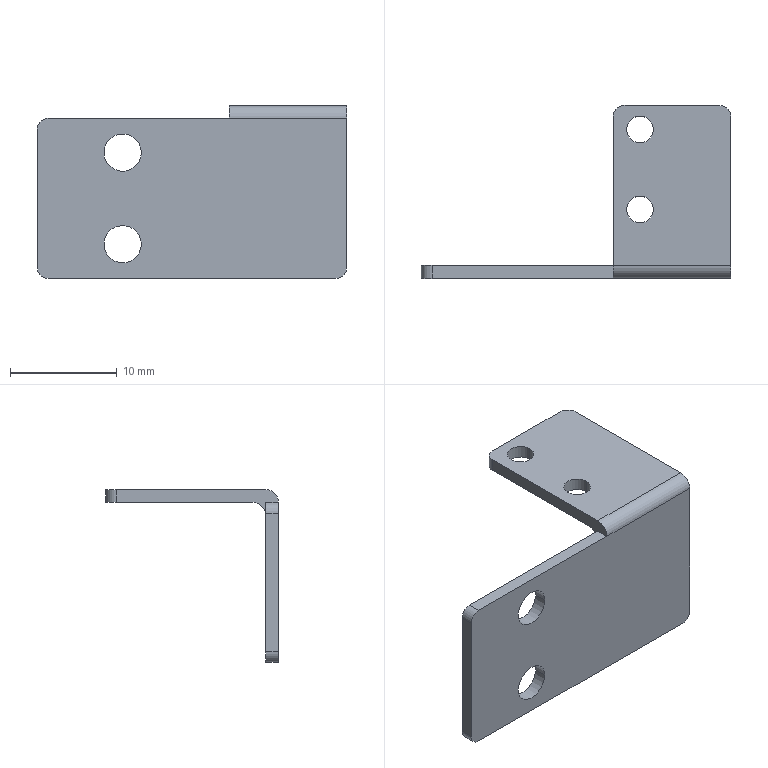Part | STEP file | 11-FG-B01311 | 1 solid | 25 faces | box 29 x 16.2 x 16.2 mm | volume 699.681 mm3 | cylinder 15 | plane 10 | commonest cylinder face diameters 2 x5 2.5 x4 3.5 x4 2.4 x2
STEP:
#1=CARTESIAN_POINT('',(-19.25,0.,-3.2));
#2=VERTEX_POINT('',#1);
#3=CARTESIAN_POINT('',(-22.75,0.,-3.2));
#4=VERTEX_POINT('',#3);
#5=CARTESIAN_POINT('',(-21.,0.,-3.2));
#6=DIRECTION('',(0.,1.,0.));
#7=DIRECTION('',(0.,0.,1.));
#8=AXIS2_PLACEMENT_3D('',#5,#6,#7);
#9=CIRCLE('',#8,1.75);
#10=EDGE_CURVE('',#2,#4,#9,.T.);
#11=ORIENTED_EDGE('',*,*,#10,.F.);
#12=CARTESIAN_POINT('',(-19.25,1.2,-3.2));
#13=VERTEX_POINT('',#12);
#14=CARTESIAN_POINT('',(-19.25,-8.8,-3.2));
#15=DIRECTION('',(0.,1.,0.));
#16=VECTOR('',#15,1000.);
#17=LINE('',#14,#16);
#18=EDGE_CURVE('',#2,#13,#17,.T.);
#19=ORIENTED_EDGE('',*,*,#18,.T.);
#20=CARTESIAN_POINT('',(-22.75,1.2,-3.2));
#21=VERTEX_POINT('',#20);
#22=CARTESIAN_POINT('',(-21.,1.2,-3.2));
#23=DIRECTION('',(0.,1.,0.));
#24=DIRECTION('',(-1.,0.,0.));
#25=AXIS2_PLACEMENT_3D('',#22,#23,#24);
#26=CIRCLE('',#25,1.75);
#27=EDGE_CURVE('',#13,#21,#26,.T.);
#28=ORIENTED_EDGE('',*,*,#27,.T.);
#29=CARTESIAN_POINT('',(-22.75,-8.8,-3.2));
#30=DIRECTION('',(0.,1.,0.));
#31=VECTOR('',#30,1000.);
#32=LINE('',#29,#31);
#33=EDGE_CURVE('',#4,#21,#32,.T.);
#34=ORIENTED_EDGE('',*,*,#33,.F.);
#35=EDGE_LOOP('',(#11,#19,#28,#34));
#36=FACE_OUTER_BOUND('',#35,.T.);
#37=CARTESIAN_POINT('',(-21.,-8.8,-3.2));
#38=DIRECTION('',(0.,1.,0.));
#39=DIRECTION('',(-1.,0.,0.));
#40=AXIS2_PLACEMENT_3D('',#37,#38,#39);
#41=CYLINDRICAL_SURFACE('',#40,1.75);
#42=ADVANCED_FACE('',(#36),#41,.F.);
#43=CARTESIAN_POINT('',(-19.25,0.,-11.8));
#44=VERTEX_POINT('',#43);
#45=CARTESIAN_POINT('',(-22.75,0.,-11.8));
#46=VERTEX_POINT('',#45);
#47=CARTESIAN_POINT('',(-21.,0.,-11.8));
#48=DIRECTION('',(0.,1.,0.));
#49=DIRECTION('',(0.,0.,1.));
#50=AXIS2_PLACEMENT_3D('',#47,#48,#49);
#51=CIRCLE('',#50,1.75);
#52=EDGE_CURVE('',#44,#46,#51,.T.);
#53=ORIENTED_EDGE('',*,*,#52,.F.);
#54=CARTESIAN_POINT('',(-19.25,1.2,-11.8));
#55=VERTEX_POINT('',#54);
#56=CARTESIAN_POINT('',(-19.25,-8.8,-11.8));
#57=DIRECTION('',(0.,1.,0.));
#58=VECTOR('',#57,1000.);
#59=LINE('',#56,#58);
#60=EDGE_CURVE('',#44,#55,#59,.T.);
#61=ORIENTED_EDGE('',*,*,#60,.T.);
#62=CARTESIAN_POINT('',(-22.75,1.2,-11.8));
#63=VERTEX_POINT('',#62);
#64=CARTESIAN_POINT('',(-21.,1.2,-11.8));
#65=DIRECTION('',(0.,1.,0.));
#66=DIRECTION('',(-1.,0.,0.));
#67=AXIS2_PLACEMENT_3D('',#64,#65,#66);
#68=CIRCLE('',#67,1.75);
#69=EDGE_CURVE('',#55,#63,#68,.T.);
#70=ORIENTED_EDGE('',*,*,#69,.T.);
#71=CARTESIAN_POINT('',(-22.75,-8.8,-11.8));
#72=DIRECTION('',(0.,1.,0.));
#73=VECTOR('',#72,1000.);
#74=LINE('',#71,#73);
#75=EDGE_CURVE('',#46,#63,#74,.T.);
#76=ORIENTED_EDGE('',*,*,#75,.F.);
#77=EDGE_LOOP('',(#53,#61,#70,#76));
#78=FACE_OUTER_BOUND('',#77,.T.);
#79=CARTESIAN_POINT('',(-21.,-8.8,-11.8));
#80=DIRECTION('',(0.,1.,0.));
#81=DIRECTION('',(-1.,0.,0.));
#82=AXIS2_PLACEMENT_3D('',#79,#80,#81);
#83=CYLINDRICAL_SURFACE('',#82,1.75);
#84=ADVANCED_FACE('',(#78),#83,.F.);
#85=CARTESIAN_POINT('',(-9.75,13.95,0.));
#86=VERTEX_POINT('',#85);
#87=CARTESIAN_POINT('',(-7.25,13.95,0.));
#88=VERTEX_POINT('',#87);
#89=CARTESIAN_POINT('',(-8.5,13.95,0.));
#90=DIRECTION('',(0.,0.,1.));
#91=DIRECTION('',(1.,0.,0.));
#92=AXIS2_PLACEMENT_3D('',#89,#90,#91);
#93=CIRCLE('',#92,1.25);
#94=EDGE_CURVE('',#86,#88,#93,.T.);
#95=ORIENTED_EDGE('',*,*,#94,.F.);
#96=CARTESIAN_POINT('',(-9.75,13.95,1.2));
#97=VERTEX_POINT('',#96);
#98=CARTESIAN_POINT('',(-9.75,13.95,1.2));
#99=DIRECTION('',(0.,0.,1.));
#100=VECTOR('',#99,1000.);
#101=LINE('',#98,#100);
#102=EDGE_CURVE('',#86,#97,#101,.T.);
#103=ORIENTED_EDGE('',*,*,#102,.T.);
#104=CARTESIAN_POINT('',(-7.25,13.95,1.2));
#105=VERTEX_POINT('',#104);
#106=CARTESIAN_POINT('',(-8.5,13.95,1.2));
#107=DIRECTION('',(0.,0.,1.));
#108=DIRECTION('',(1.,0.,0.));
#109=AXIS2_PLACEMENT_3D('',#106,#107,#108);
#110=CIRCLE('',#109,1.25);
#111=EDGE_CURVE('',#97,#105,#110,.T.);
#112=ORIENTED_EDGE('',*,*,#111,.T.);
#113=CARTESIAN_POINT('',(-7.25,13.95,1.2));
#114=DIRECTION('',(0.,0.,1.));
#115=VECTOR('',#114,1000.);
#116=LINE('',#113,#115);
#117=EDGE_CURVE('',#88,#105,#116,.T.);
#118=ORIENTED_EDGE('',*,*,#117,.F.);
#119=EDGE_LOOP('',(#95,#103,#112,#118));
#120=FACE_OUTER_BOUND('',#119,.T.);
#121=CARTESIAN_POINT('',(-8.5,13.95,1.2));
#122=DIRECTION('',(0.,0.,1.));
#123=DIRECTION('',(1.,0.,0.));
#124=AXIS2_PLACEMENT_3D('',#121,#122,#123);
#125=CYLINDRICAL_SURFACE('',#124,1.25);
#126=ADVANCED_FACE('',(#120),#125,.F.);
#127=CARTESIAN_POINT('',(-9.75,6.45,0.));
#128=VERTEX_POINT('',#127);
#129=CARTESIAN_POINT('',(-7.25,6.45,0.));
#130=VERTEX_POINT('',#129);
#131=CARTESIAN_POINT('',(-8.5,6.45,0.));
#132=DIRECTION('',(0.,0.,1.));
#133=DIRECTION('',(1.,0.,0.));
#134=AXIS2_PLACEMENT_3D('',#131,#132,#133);
#135=CIRCLE('',#134,1.25);
#136=EDGE_CURVE('',#128,#130,#135,.T.);
#137=ORIENTED_EDGE('',*,*,#136,.F.);
#138=CARTESIAN_POINT('',(-9.75,6.45,1.2));
#139=VERTEX_POINT('',#138);
#140=CARTESIAN_POINT('',(-9.75,6.45,1.2));
#141=DIRECTION('',(0.,0.,1.));
#142=VECTOR('',#141,1000.);
#143=LINE('',#140,#142);
#144=EDGE_CURVE('',#128,#139,#143,.T.);
#145=ORIENTED_EDGE('',*,*,#144,.T.);
#146=CARTESIAN_POINT('',(-7.25,6.45,1.2));
#147=VERTEX_POINT('',#146);
#148=CARTESIAN_POINT('',(-8.5,6.45,1.2));
#149=DIRECTION('',(0.,0.,1.));
#150=DIRECTION('',(1.,0.,0.));
#151=AXIS2_PLACEMENT_3D('',#148,#149,#150);
#152=CIRCLE('',#151,1.25);
#153=EDGE_CURVE('',#139,#147,#152,.T.);
#154=ORIENTED_EDGE('',*,*,#153,.T.);
#155=CARTESIAN_POINT('',(-7.25,6.45,1.2));
#156=DIRECTION('',(0.,0.,1.));
#157=VECTOR('',#156,1000.);
#158=LINE('',#155,#157);
#159=EDGE_CURVE('',#130,#147,#158,.T.);
#160=ORIENTED_EDGE('',*,*,#159,.F.);
#161=EDGE_LOOP('',(#137,#145,#154,#160));
#162=FACE_OUTER_BOUND('',#161,.T.);
#163=CARTESIAN_POINT('',(-8.5,6.45,1.2));
#164=DIRECTION('',(0.,0.,1.));
#165=DIRECTION('',(1.,0.,0.));
#166=AXIS2_PLACEMENT_3D('',#163,#164,#165);
#167=CYLINDRICAL_SURFACE('',#166,1.25);
#168=ADVANCED_FACE('',(#162),#167,.F.);
#169=CARTESIAN_POINT('',(-8.5,13.95,0.));
#170=DIRECTION('',(0.,0.,1.));
#171=DIRECTION('',(1.,0.,0.));
#172=AXIS2_PLACEMENT_3D('',#169,#170,#171);
#173=CIRCLE('',#172,1.25);
#174=EDGE_CURVE('',#88,#86,#173,.T.);
#175=ORIENTED_EDGE('',*,*,#174,.T.);
#176=ORIENTED_EDGE('',*,*,#94,.T.);
#177=EDGE_LOOP('',(#175,#176));
#178=FACE_BOUND('',#177,.T.);
#179=CARTESIAN_POINT('',(-8.5,6.45,0.));
#180=DIRECTION('',(0.,0.,1.));
#181=DIRECTION('',(1.,0.,0.));
#182=AXIS2_PLACEMENT_3D('',#179,#180,#181);
#183=CIRCLE('',#182,1.25);
#184=EDGE_CURVE('',#130,#128,#183,.T.);
#185=ORIENTED_EDGE('',*,*,#184,.T.);
#186=ORIENTED_EDGE('',*,*,#136,.T.);
#187=EDGE_LOOP('',(#185,#186));
#188=FACE_BOUND('',#187,.T.);
#189=CARTESIAN_POINT('',(-1.,16.2,0.));
#190=VERTEX_POINT('',#189);
#191=CARTESIAN_POINT('',(-10.,16.2,0.));
#192=VERTEX_POINT('',#191);
#193=CARTESIAN_POINT('',(-11.,16.2,0.));
#194=DIRECTION('',(-1.,0.,0.));
#195=VECTOR('',#194,1000.);
#196=LINE('',#193,#195);
#197=EDGE_CURVE('',#190,#192,#196,.T.);
#198=ORIENTED_EDGE('',*,*,#197,.F.);
#199=CARTESIAN_POINT('',(0.,15.2,0.));
#200=VERTEX_POINT('',#199);
#201=CARTESIAN_POINT('',(-1.,15.2,0.));
#202=DIRECTION('',(0.,0.,-1.));
#203=DIRECTION('',(1.,0.,0.));
#204=AXIS2_PLACEMENT_3D('',#201,#202,#203);
#205=CIRCLE('',#204,1.);
#206=EDGE_CURVE('',#190,#200,#205,.T.);
#207=ORIENTED_EDGE('',*,*,#206,.T.);
#208=CARTESIAN_POINT('',(0.,2.4,0.));
#209=VERTEX_POINT('',#208);
#210=CARTESIAN_POINT('',(0.,16.2,0.));
#211=DIRECTION('',(0.,1.,0.));
#212=VECTOR('',#211,1000.);
#213=LINE('',#210,#212);
#214=EDGE_CURVE('',#209,#200,#213,.T.);
#215=ORIENTED_EDGE('',*,*,#214,.F.);
#216=CARTESIAN_POINT('',(-11.,2.4,0.));
#217=VERTEX_POINT('',#216);
#218=CARTESIAN_POINT('',(-11.,2.4,0.));
#219=DIRECTION('',(-1.,0.,0.));
#220=VECTOR('',#219,1000.);
#221=LINE('',#218,#220);
#222=EDGE_CURVE('',#209,#217,#221,.T.);
#223=ORIENTED_EDGE('',*,*,#222,.T.);
#224=CARTESIAN_POINT('',(-11.,15.2,0.));
#225=VERTEX_POINT('',#224);
#226=CARTESIAN_POINT('',(-11.,16.2,0.));
#227=DIRECTION('',(0.,-1.,0.));
#228=VECTOR('',#227,1000.);
#229=LINE('',#226,#228);
#230=EDGE_CURVE('',#225,#217,#229,.T.);
#231=ORIENTED_EDGE('',*,*,#230,.F.);
#232=CARTESIAN_POINT('',(-10.,15.2,0.));
#233=DIRECTION('',(0.,0.,-1.));
#234=DIRECTION('',(1.,0.,0.));
#235=AXIS2_PLACEMENT_3D('',#232,#233,#234);
#236=CIRCLE('',#235,1.);
#237=EDGE_CURVE('',#225,#192,#236,.T.);
#238=ORIENTED_EDGE('',*,*,#237,.T.);
#239=EDGE_LOOP('',(#198,#207,#215,#223,#231,#238));
#240=FACE_OUTER_BOUND('',#239,.T.);
#241=CARTESIAN_POINT('',(-11.,0.,0.));
#242=DIRECTION('',(0.,0.,1.));
#243=DIRECTION('',(1.,0.,0.));
#244=AXIS2_PLACEMENT_3D('',#241,#242,#243);
#245=PLANE('',#244);
#246=ADVANCED_FACE('',(#178,#188,#240),#245,.F.);
#247=CARTESIAN_POINT('',(-11.,15.2,1.2));
#248=VERTEX_POINT('',#247);
#249=CARTESIAN_POINT('',(-11.,1.2,1.2));
#250=VERTEX_POINT('',#249);
#251=CARTESIAN_POINT('',(-11.,16.2,1.2));
#252=DIRECTION('',(0.,-1.,0.));
#253=VECTOR('',#252,1000.);
#254=LINE('',#251,#253);
#255=EDGE_CURVE('',#248,#250,#254,.T.);
#256=ORIENTED_EDGE('',*,*,#255,.F.);
#257=CARTESIAN_POINT('',(-11.,15.2,1.2));
#258=DIRECTION('',(0.,0.,-1.));
#259=VECTOR('',#258,1000.);
#260=LINE('',#257,#259);
#261=EDGE_CURVE('',#248,#225,#260,.T.);
#262=ORIENTED_EDGE('',*,*,#261,.T.);
#263=ORIENTED_EDGE('',*,*,#230,.T.);
#264=CARTESIAN_POINT('',(-11.,1.2,-1.2));
#265=VERTEX_POINT('',#264);
#266=CARTESIAN_POINT('',(-11.,2.4,-1.2));
#267=DIRECTION('',(1.,0.,0.));
#268=DIRECTION('',(0.,1.,0.));
#269=AXIS2_PLACEMENT_3D('',#266,#267,#268);
#270=CIRCLE('',#269,1.2);
#271=EDGE_CURVE('',#217,#265,#270,.T.);
#272=ORIENTED_EDGE('',*,*,#271,.T.);
#273=CARTESIAN_POINT('',(-11.,1.2,0.));
#274=VERTEX_POINT('',#273);
#275=CARTESIAN_POINT('',(-11.,1.2,0.));
#276=DIRECTION('',(0.,0.,-1.));
#277=VECTOR('',#276,1000.);
#278=LINE('',#275,#277);
#279=EDGE_CURVE('',#274,#265,#278,.T.);
#280=ORIENTED_EDGE('',*,*,#279,.F.);
#281=CARTESIAN_POINT('',(-11.,0.,0.));
#282=VERTEX_POINT('',#281);
#283=CARTESIAN_POINT('',(-11.,16.2,0.));
#284=DIRECTION('',(0.,-1.,0.));
#285=VECTOR('',#284,1000.);
#286=LINE('',#283,#285);
#287=EDGE_CURVE('',#274,#282,#286,.T.);
#288=ORIENTED_EDGE('',*,*,#287,.T.);
#289=CARTESIAN_POINT('',(-11.,1.2,0.));
#290=DIRECTION('',(-1.,0.,0.));
#291=DIRECTION('',(0.,1.,0.));
#292=AXIS2_PLACEMENT_3D('',#289,#290,#291);
#293=CIRCLE('',#292,1.2);
#294=EDGE_CURVE('',#282,#250,#293,.T.);
#295=ORIENTED_EDGE('',*,*,#294,.T.);
#296=EDGE_LOOP('',(#256,#262,#263,#272,#280,#288,#295));
#297=FACE_OUTER_BOUND('',#296,.T.);
#298=CARTESIAN_POINT('',(-11.,16.2,1.2));
#299=DIRECTION('',(1.,0.,0.));
#300=DIRECTION('',(0.,1.,0.));
#301=AXIS2_PLACEMENT_3D('',#298,#299,#300);
#302=PLANE('',#301);
#303=ADVANCED_FACE('',(#297),#302,.F.);
#304=CARTESIAN_POINT('',(-21.,0.,-3.2));
#305=DIRECTION('',(0.,1.,0.));
#306=DIRECTION('',(0.,0.,1.));
#307=AXIS2_PLACEMENT_3D('',#304,#305,#306);
#308=CIRCLE('',#307,1.75);
#309=EDGE_CURVE('',#4,#2,#308,.T.);
#310=ORIENTED_EDGE('',*,*,#309,.T.);
#311=ORIENTED_EDGE('',*,*,#10,.T.);
#312=EDGE_LOOP('',(#310,#311));
#313=FACE_BOUND('',#312,.T.);
#314=CARTESIAN_POINT('',(-21.,0.,-11.8));
#315=DIRECTION('',(0.,1.,0.));
#316=DIRECTION('',(0.,0.,1.));
#317=AXIS2_PLACEMENT_3D('',#314,#315,#316);
#318=CIRCLE('',#317,1.75);
#319=EDGE_CURVE('',#46,#44,#318,.T.);
#320=ORIENTED_EDGE('',*,*,#319,.T.);
#321=ORIENTED_EDGE('',*,*,#52,.T.);
#322=EDGE_LOOP('',(#320,#321));
#323=FACE_BOUND('',#322,.T.);
#324=CARTESIAN_POINT('',(-28.,0.,0.));
#325=VERTEX_POINT('',#324);
#326=CARTESIAN_POINT('',(-29.,0.,0.));
#327=DIRECTION('',(1.,0.,0.));
#328=VECTOR('',#327,1000.);
#329=LINE('',#326,#328);
#330=EDGE_CURVE('',#325,#282,#329,.T.);
#331=ORIENTED_EDGE('',*,*,#330,.F.);
#332=CARTESIAN_POINT('',(-29.,0.,-1.));
#333=VERTEX_POINT('',#332);
#334=CARTESIAN_POINT('',(-28.,0.,-1.));
#335=DIRECTION('',(0.,-1.,0.));
#336=DIRECTION('',(0.,0.,1.));
#337=AXIS2_PLACEMENT_3D('',#334,#335,#336);
#338=CIRCLE('',#337,1.);
#339=EDGE_CURVE('',#325,#333,#338,.T.);
#340=ORIENTED_EDGE('',*,*,#339,.T.);
#341=CARTESIAN_POINT('',(-29.,0.,-14.));
#342=VERTEX_POINT('',#341);
#343=CARTESIAN_POINT('',(-29.,0.,0.));
#344=DIRECTION('',(0.,0.,-1.));
#345=VECTOR('',#344,1000.);
#346=LINE('',#343,#345);
#347=EDGE_CURVE('',#333,#342,#346,.T.);
#348=ORIENTED_EDGE('',*,*,#347,.T.);
#349=CARTESIAN_POINT('',(-28.,0.,-15.));
#350=VERTEX_POINT('',#349);
#351=CARTESIAN_POINT('',(-28.,0.,-14.));
#352=DIRECTION('',(0.,-1.,0.));
#353=DIRECTION('',(0.,0.,1.));
#354=AXIS2_PLACEMENT_3D('',#351,#352,#353);
#355=CIRCLE('',#354,1.);
#356=EDGE_CURVE('',#342,#350,#355,.T.);
#357=ORIENTED_EDGE('',*,*,#356,.T.);
#358=CARTESIAN_POINT('',(-1.,0.,-15.));
#359=VERTEX_POINT('',#358);
#360=CARTESIAN_POINT('',(-29.,0.,-15.));
#361=DIRECTION('',(1.,0.,0.));
#362=VECTOR('',#361,1000.);
#363=LINE('',#360,#362);
#364=EDGE_CURVE('',#350,#359,#363,.T.);
#365=ORIENTED_EDGE('',*,*,#364,.T.);
#366=CARTESIAN_POINT('',(0.,0.,-14.));
#367=VERTEX_POINT('',#366);
#368=CARTESIAN_POINT('',(-1.,0.,-14.));
#369=DIRECTION('',(0.,-1.,0.));
#370=DIRECTION('',(0.,0.,1.));
#371=AXIS2_PLACEMENT_3D('',#368,#369,#370);
#372=CIRCLE('',#371,1.);
#373=EDGE_CURVE('',#359,#367,#372,.T.);
#374=ORIENTED_EDGE('',*,*,#373,.T.);
#375=CARTESIAN_POINT('',(0.,0.,0.));
#376=VERTEX_POINT('',#375);
#377=CARTESIAN_POINT('',(0.,0.,1.2));
#378=DIRECTION('',(0.,0.,-1.));
#379=VECTOR('',#378,1000.);
#380=LINE('',#377,#379);
#381=EDGE_CURVE('',#376,#367,#380,.T.);
#382=ORIENTED_EDGE('',*,*,#381,.F.);
#383=CARTESIAN_POINT('',(-11.,0.,0.));
#384=DIRECTION('',(-1.,0.,0.));
#385=VECTOR('',#384,1000.);
#386=LINE('',#383,#385);
#387=EDGE_CURVE('',#376,#282,#386,.T.);
#388=ORIENTED_EDGE('',*,*,#387,.T.);
#389=EDGE_LOOP('',(#331,#340,#348,#357,#365,#374,#382,#388));
#390=FACE_OUTER_BOUND('',#389,.T.);
#391=CARTESIAN_POINT('',(-11.,0.,1.2));
#392=DIRECTION('',(0.,1.,0.));
#393=DIRECTION('',(0.,0.,1.));
#394=AXIS2_PLACEMENT_3D('',#391,#392,#393);
#395=PLANE('',#394);
#396=ADVANCED_FACE('',(#313,#323,#390),#395,.F.);
#397=ORIENTED_EDGE('',*,*,#381,.T.);
#398=CARTESIAN_POINT('',(0.,1.2,-14.));
#399=VERTEX_POINT('',#398);
#400=CARTESIAN_POINT('',(0.,1.2,-14.));
#401=DIRECTION('',(0.,1.,0.));
#402=VECTOR('',#401,1000.);
#403=LINE('',#400,#402);
#404=EDGE_CURVE('',#367,#399,#403,.T.);
#405=ORIENTED_EDGE('',*,*,#404,.T.);
#406=CARTESIAN_POINT('',(0.,1.2,-1.2));
#407=VERTEX_POINT('',#406);
#408=CARTESIAN_POINT('',(0.,1.2,0.));
#409=DIRECTION('',(0.,0.,1.));
#410=VECTOR('',#409,1000.);
#411=LINE('',#408,#410);
#412=EDGE_CURVE('',#399,#407,#411,.T.);
#413=ORIENTED_EDGE('',*,*,#412,.T.);
#414=CARTESIAN_POINT('',(0.,2.4,-1.2));
#415=DIRECTION('',(-1.,0.,0.));
#416=DIRECTION('',(0.,-1.,0.));
#417=AXIS2_PLACEMENT_3D('',#414,#415,#416);
#418=CIRCLE('',#417,1.2);
#419=EDGE_CURVE('',#407,#209,#418,.T.);
#420=ORIENTED_EDGE('',*,*,#419,.T.);
#421=ORIENTED_EDGE('',*,*,#214,.T.);
#422=CARTESIAN_POINT('',(0.,15.2,1.2));
#423=VERTEX_POINT('',#422);
#424=CARTESIAN_POINT('',(0.,15.2,1.2));
#425=DIRECTION('',(0.,0.,1.));
#426=VECTOR('',#425,1000.);
#427=LINE('',#424,#426);
#428=EDGE_CURVE('',#200,#423,#427,.T.);
#429=ORIENTED_EDGE('',*,*,#428,.T.);
#430=CARTESIAN_POINT('',(0.,1.2,1.2));
#431=VERTEX_POINT('',#430);
#432=CARTESIAN_POINT('',(0.,16.2,1.2));
#433=DIRECTION('',(0.,1.,0.));
#434=VECTOR('',#433,1000.);
#435=LINE('',#432,#434);
#436=EDGE_CURVE('',#431,#423,#435,.T.);
#437=ORIENTED_EDGE('',*,*,#436,.F.);
#438=CARTESIAN_POINT('',(0.,1.2,0.));
#439=DIRECTION('',(1.,0.,0.));
#440=DIRECTION('',(0.,-1.,0.));
#441=AXIS2_PLACEMENT_3D('',#438,#439,#440);
#442=CIRCLE('',#441,1.2);
#443=EDGE_CURVE('',#431,#376,#442,.T.);
#444=ORIENTED_EDGE('',*,*,#443,.T.);
#445=EDGE_LOOP('',(#397,#405,#413,#420,#421,#429,#437,#444));
#446=FACE_OUTER_BOUND('',#445,.T.);
#447=CARTESIAN_POINT('',(0.,16.2,1.2));
#448=DIRECTION('',(-1.,0.,0.));
#449=DIRECTION('',(0.,-1.,0.));
#450=AXIS2_PLACEMENT_3D('',#447,#448,#449);
#451=PLANE('',#450);
#452=ADVANCED_FACE('',(#446),#451,.F.);
#453=CARTESIAN_POINT('',(-1.,16.2,1.2));
#454=VERTEX_POINT('',#453);
#455=CARTESIAN_POINT('',(-10.,16.2,1.2));
#456=VERTEX_POINT('',#455);
#457=CARTESIAN_POINT('',(-11.,16.2,1.2));
#458=DIRECTION('',(-1.,0.,0.));
#459=VECTOR('',#458,1000.);
#460=LINE('',#457,#459);
#461=EDGE_CURVE('',#454,#456,#460,.T.);
#462=ORIENTED_EDGE('',*,*,#461,.F.);
#463=CARTESIAN_POINT('',(-1.,16.2,1.2));
#464=DIRECTION('',(0.,0.,-1.));
#465=VECTOR('',#464,1000.);
#466=LINE('',#463,#465);
#467=EDGE_CURVE('',#454,#190,#466,.T.);
#468=ORIENTED_EDGE('',*,*,#467,.T.);
#469=ORIENTED_EDGE('',*,*,#197,.T.);
#470=CARTESIAN_POINT('',(-10.,16.2,1.2));
#471=DIRECTION('',(0.,0.,1.));
#472=VECTOR('',#471,1000.);
#473=LINE('',#470,#472);
#474=EDGE_CURVE('',#192,#456,#473,.T.);
#475=ORIENTED_EDGE('',*,*,#474,.T.);
#476=EDGE_LOOP('',(#462,#468,#469,#475));
#477=FACE_OUTER_BOUND('',#476,.T.);
#478=CARTESIAN_POINT('',(-11.,16.2,1.2));
#479=DIRECTION('',(0.,-1.,0.));
#480=DIRECTION('',(0.,0.,-1.));
#481=AXIS2_PLACEMENT_3D('',#478,#479,#480);
#482=PLANE('',#481);
#483=ADVANCED_FACE('',(#477),#482,.F.);
#484=CARTESIAN_POINT('',(-8.5,13.95,1.2));
#485=DIRECTION('',(0.,0.,1.));
#486=DIRECTION('',(1.,0.,0.));
#487=AXIS2_PLACEMENT_3D('',#484,#485,#486);
#488=CIRCLE('',#487,1.25);
#489=EDGE_CURVE('',#105,#97,#488,.T.);
#490=ORIENTED_EDGE('',*,*,#489,.F.);
#491=ORIENTED_EDGE('',*,*,#111,.F.);
#492=EDGE_LOOP('',(#490,#491));
#493=FACE_BOUND('',#492,.T.);
#494=CARTESIAN_POINT('',(-8.5,6.45,1.2));
#495=DIRECTION('',(0.,0.,1.));
#496=DIRECTION('',(1.,0.,0.));
#497=AXIS2_PLACEMENT_3D('',#494,#495,#496);
#498=CIRCLE('',#497,1.25);
#499=EDGE_CURVE('',#147,#139,#498,.T.);
#500=ORIENTED_EDGE('',*,*,#499,.F.);
#501=ORIENTED_EDGE('',*,*,#153,.F.);
#502=EDGE_LOOP('',(#500,#501));
#503=FACE_BOUND('',#502,.T.);
#504=ORIENTED_EDGE('',*,*,#436,.T.);
#505=CARTESIAN_POINT('',(-1.,15.2,1.2));
#506=DIRECTION('',(0.,0.,1.));
#507=DIRECTION('',(1.,0.,0.));
#508=AXIS2_PLACEMENT_3D('',#505,#506,#507);
#509=CIRCLE('',#508,1.);
#510=EDGE_CURVE('',#423,#454,#509,.T.);
#511=ORIENTED_EDGE('',*,*,#510,.T.);
#512=ORIENTED_EDGE('',*,*,#461,.T.);
#513=CARTESIAN_POINT('',(-10.,15.2,1.2));
#514=DIRECTION('',(0.,0.,1.));
#515=DIRECTION('',(1.,0.,0.));
#516=AXIS2_PLACEMENT_3D('',#513,#514,#515);
#517=CIRCLE('',#516,1.);
#518=EDGE_CURVE('',#456,#248,#517,.T.);
#519=ORIENTED_EDGE('',*,*,#518,.T.);
#520=ORIENTED_EDGE('',*,*,#255,.T.);
#521=CARTESIAN_POINT('',(0.,1.2,1.2));
#522=DIRECTION('',(1.,0.,0.));
#523=VECTOR('',#522,1000.);
#524=LINE('',#521,#523);
#525=EDGE_CURVE('',#250,#431,#524,.T.);
#526=ORIENTED_EDGE('',*,*,#525,.T.);
#527=EDGE_LOOP('',(#504,#511,#512,#519,#520,#526));
#528=FACE_OUTER_BOUND('',#527,.T.);
#529=CARTESIAN_POINT('',(-11.,0.,1.2));
#530=DIRECTION('',(0.,0.,1.));
#531=DIRECTION('',(1.,0.,0.));
#532=AXIS2_PLACEMENT_3D('',#529,#530,#531);
#533=PLANE('',#532);
#534=ADVANCED_FACE('',(#493,#503,#528),#533,.T.);
#535=CARTESIAN_POINT('',(-28.,1.2,0.));
#536=VERTEX_POINT('',#535);
#537=CARTESIAN_POINT('',(-29.,1.2,0.));
#538=DIRECTION('',(1.,0.,0.));
#539=VECTOR('',#538,1000.);
#540=LINE('',#537,#539);
#541=EDGE_CURVE('',#536,#274,#540,.T.);
#542=ORIENTED_EDGE('',*,*,#541,.F.);
#543=CARTESIAN_POINT('',(-28.,0.,0.));
#544=DIRECTION('',(0.,-1.,0.));
#545=VECTOR('',#544,1000.);
#546=LINE('',#543,#545);
#547=EDGE_CURVE('',#536,#325,#546,.T.);
#548=ORIENTED_EDGE('',*,*,#547,.T.);
#549=ORIENTED_EDGE('',*,*,#330,.T.);
#550=ORIENTED_EDGE('',*,*,#287,.F.);
#551=EDGE_LOOP('',(#542,#548,#549,#550));
#552=FACE_OUTER_BOUND('',#551,.T.);
#553=CARTESIAN_POINT('',(-29.,0.,0.));
#554=DIRECTION('',(0.,0.,1.));
#555=DIRECTION('',(1.,0.,0.));
#556=AXIS2_PLACEMENT_3D('',#553,#554,#555);
#557=PLANE('',#556);
#558=ADVANCED_FACE('',(#552),#557,.T.);
#559=CARTESIAN_POINT('',(-21.,1.2,-3.2));
#560=DIRECTION('',(0.,1.,0.));
#561=DIRECTION('',(-1.,0.,0.));
#562=AXIS2_PLACEMENT_3D('',#559,#560,#561);
#563=CIRCLE('',#562,1.75);
#564=EDGE_CURVE('',#21,#13,#563,.T.);
#565=ORIENTED_EDGE('',*,*,#564,.F.);
#566=ORIENTED_EDGE('',*,*,#27,.F.);
#567=EDGE_LOOP('',(#565,#566));
#568=FACE_BOUND('',#567,.T.);
#569=CARTESIAN_POINT('',(-21.,1.2,-11.8));
#570=DIRECTION('',(0.,1.,0.));
#571=DIRECTION('',(-1.,0.,0.));
#572=AXIS2_PLACEMENT_3D('',#569,#570,#571);
#573=CIRCLE('',#572,1.75);
#574=EDGE_CURVE('',#63,#55,#573,.T.);
#575=ORIENTED_EDGE('',*,*,#574,.F.);
#576=ORIENTED_EDGE('',*,*,#69,.F.);
#577=EDGE_LOOP('',(#575,#576));
#578=FACE_BOUND('',#577,.T.);
#579=CARTESIAN_POINT('',(-29.,1.2,-14.));
#580=VERTEX_POINT('',#579);
#581=CARTESIAN_POINT('',(-29.,1.2,-1.));
#582=VERTEX_POINT('',#581);
#583=CARTESIAN_POINT('',(-29.,1.2,0.));
#584=DIRECTION('',(0.,0.,1.));
#585=VECTOR('',#584,1000.);
#586=LINE('',#583,#585);
#587=EDGE_CURVE('',#580,#582,#586,.T.);
#588=ORIENTED_EDGE('',*,*,#587,.T.);
#589=CARTESIAN_POINT('',(-28.,1.2,-1.));
#590=DIRECTION('',(0.,1.,0.));
#591=DIRECTION('',(-1.,0.,0.));
#592=AXIS2_PLACEMENT_3D('',#589,#590,#591);
#593=CIRCLE('',#592,1.);
#594=EDGE_CURVE('',#582,#536,#593,.T.);
#595=ORIENTED_EDGE('',*,*,#594,.T.);
#596=ORIENTED_EDGE('',*,*,#541,.T.);
#597=ORIENTED_EDGE('',*,*,#279,.T.);
#598=CARTESIAN_POINT('',(-29.,1.2,-1.2));
#599=DIRECTION('',(1.,0.,0.));
#600=VECTOR('',#599,1000.);
#601=LINE('',#598,#600);
#602=EDGE_CURVE('',#265,#407,#601,.T.);
#603=ORIENTED_EDGE('',*,*,#602,.T.);
#604=ORIENTED_EDGE('',*,*,#412,.F.);
#605=CARTESIAN_POINT('',(-1.,1.2,-15.));
#606=VERTEX_POINT('',#605);
#607=CARTESIAN_POINT('',(-1.,1.2,-14.));
#608=DIRECTION('',(0.,1.,0.));
#609=DIRECTION('',(-1.,0.,0.));
#610=AXIS2_PLACEMENT_3D('',#607,#608,#609);
#611=CIRCLE('',#610,1.);
#612=EDGE_CURVE('',#399,#606,#611,.T.);
#613=ORIENTED_EDGE('',*,*,#612,.T.);
#614=CARTESIAN_POINT('',(-28.,1.2,-15.));
#615=VERTEX_POINT('',#614);
#616=CARTESIAN_POINT('',(-29.,1.2,-15.));
#617=DIRECTION('',(1.,0.,0.));
#618=VECTOR('',#617,1000.);
#619=LINE('',#616,#618);
#620=EDGE_CURVE('',#615,#606,#619,.T.);
#621=ORIENTED_EDGE('',*,*,#620,.F.);
#622=CARTESIAN_POINT('',(-28.,1.2,-14.));
#623=DIRECTION('',(0.,1.,0.));
#624=DIRECTION('',(-1.,0.,0.));
#625=AXIS2_PLACEMENT_3D('',#622,#623,#624);
#626=CIRCLE('',#625,1.);
#627=EDGE_CURVE('',#615,#580,#626,.T.);
#628=ORIENTED_EDGE('',*,*,#627,.T.);
#629=EDGE_LOOP('',(#588,#595,#596,#597,#603,#604,#613,#621,#628));
#630=FACE_OUTER_BOUND('',#629,.T.);
#631=CARTESIAN_POINT('',(-29.,1.2,0.));
#632=DIRECTION('',(0.,1.,0.));
#633=DIRECTION('',(-1.,0.,0.));
#634=AXIS2_PLACEMENT_3D('',#631,#632,#633);
#635=PLANE('',#634);
#636=ADVANCED_FACE('',(#568,#578,#630),#635,.T.);
#637=ORIENTED_EDGE('',*,*,#364,.F.);
#638=CARTESIAN_POINT('',(-28.,0.,-15.));
#639=DIRECTION('',(0.,1.,0.));
#640=VECTOR('',#639,1000.);
#641=LINE('',#638,#640);
#642=EDGE_CURVE('',#350,#615,#641,.T.);
#643=ORIENTED_EDGE('',*,*,#642,.T.);
#644=ORIENTED_EDGE('',*,*,#620,.T.);
#645=CARTESIAN_POINT('',(-1.,0.,-15.));
#646=DIRECTION('',(0.,-1.,0.));
#647=VECTOR('',#646,1000.);
#648=LINE('',#645,#647);
#649=EDGE_CURVE('',#606,#359,#648,.T.);
#650=ORIENTED_EDGE('',*,*,#649,.T.);
#651=EDGE_LOOP('',(#637,#643,#644,#650));
#652=FACE_OUTER_BOUND('',#651,.T.);
#653=CARTESIAN_POINT('',(-29.,0.,-15.));
#654=DIRECTION('',(0.,0.,-1.));
#655=DIRECTION('',(-1.,0.,0.));
#656=AXIS2_PLACEMENT_3D('',#653,#654,#655);
#657=PLANE('',#656);
#658=ADVANCED_FACE('',(#652),#657,.T.);
#659=ORIENTED_EDGE('',*,*,#347,.F.);
#660=CARTESIAN_POINT('',(-29.,0.,-1.));
#661=DIRECTION('',(0.,1.,0.));
#662=VECTOR('',#661,1000.);
#663=LINE('',#660,#662);
#664=EDGE_CURVE('',#333,#582,#663,.T.);
#665=ORIENTED_EDGE('',*,*,#664,.T.);
#666=ORIENTED_EDGE('',*,*,#587,.F.);
#667=CARTESIAN_POINT('',(-29.,0.,-14.));
#668=DIRECTION('',(0.,-1.,0.));
#669=VECTOR('',#668,1000.);
#670=LINE('',#667,#669);
#671=EDGE_CURVE('',#580,#342,#670,.T.);
#672=ORIENTED_EDGE('',*,*,#671,.T.);
#673=EDGE_LOOP('',(#659,#665,#666,#672));
#674=FACE_OUTER_BOUND('',#673,.T.);
#675=CARTESIAN_POINT('',(-29.,0.,0.));
#676=DIRECTION('',(-1.,0.,0.));
#677=DIRECTION('',(0.,-1.,0.));
#678=AXIS2_PLACEMENT_3D('',#675,#676,#677);
#679=PLANE('',#678);
#680=ADVANCED_FACE('',(#674),#679,.T.);
#681=ORIENTED_EDGE('',*,*,#294,.F.);
#682=ORIENTED_EDGE('',*,*,#387,.F.);
#683=ORIENTED_EDGE('',*,*,#443,.F.);
#684=ORIENTED_EDGE('',*,*,#525,.F.);
#685=EDGE_LOOP('',(#681,#682,#683,#684));
#686=FACE_OUTER_BOUND('',#685,.T.);
#687=CARTESIAN_POINT('',(-11.,1.2,0.));
#688=DIRECTION('',(-1.,0.,0.));
#689=DIRECTION('',(0.,0.,1.));
#690=AXIS2_PLACEMENT_3D('',#687,#688,#689);
#691=CYLINDRICAL_SURFACE('',#690,1.2);
#692=ADVANCED_FACE('',(#686),#691,.T.);
#693=ORIENTED_EDGE('',*,*,#271,.F.);
#694=ORIENTED_EDGE('',*,*,#222,.F.);
#695=ORIENTED_EDGE('',*,*,#419,.F.);
#696=ORIENTED_EDGE('',*,*,#602,.F.);
#697=EDGE_LOOP('',(#693,#694,#695,#696));
#698=FACE_OUTER_BOUND('',#697,.T.);
#699=CARTESIAN_POINT('',(-29.,2.4,-1.2));
#700=DIRECTION('',(1.,0.,0.));
#701=DIRECTION('',(0.,1.,0.));
#702=AXIS2_PLACEMENT_3D('',#699,#700,#701);
#703=CYLINDRICAL_SURFACE('',#702,1.2);
#704=ADVANCED_FACE('',(#698),#703,.F.);
#705=ORIENTED_EDGE('',*,*,#144,.F.);
#706=ORIENTED_EDGE('',*,*,#184,.F.);
#707=ORIENTED_EDGE('',*,*,#159,.T.);
#708=ORIENTED_EDGE('',*,*,#499,.T.);
#709=EDGE_LOOP('',(#705,#706,#707,#708));
#710=FACE_OUTER_BOUND('',#709,.T.);
#711=CARTESIAN_POINT('',(-8.5,6.45,1.2));
#712=DIRECTION('',(0.,0.,1.));
#713=DIRECTION('',(1.,0.,0.));
#714=AXIS2_PLACEMENT_3D('',#711,#712,#713);
#715=CYLINDRICAL_SURFACE('',#714,1.25);
#716=ADVANCED_FACE('',(#710),#715,.F.);
#717=ORIENTED_EDGE('',*,*,#102,.F.);
#718=ORIENTED_EDGE('',*,*,#174,.F.);
#719=ORIENTED_EDGE('',*,*,#117,.T.);
#720=ORIENTED_EDGE('',*,*,#489,.T.);
#721=EDGE_LOOP('',(#717,#718,#719,#720));
#722=FACE_OUTER_BOUND('',#721,.T.);
#723=CARTESIAN_POINT('',(-8.5,13.95,1.2));
#724=DIRECTION('',(0.,0.,1.));
#725=DIRECTION('',(1.,0.,0.));
#726=AXIS2_PLACEMENT_3D('',#723,#724,#725);
#727=CYLINDRICAL_SURFACE('',#726,1.25);
#728=ADVANCED_FACE('',(#722),#727,.F.);
#729=ORIENTED_EDGE('',*,*,#594,.F.);
#730=ORIENTED_EDGE('',*,*,#664,.F.);
#731=ORIENTED_EDGE('',*,*,#339,.F.);
#732=ORIENTED_EDGE('',*,*,#547,.F.);
#733=EDGE_LOOP('',(#729,#730,#731,#732));
#734=FACE_OUTER_BOUND('',#733,.T.);
#735=CARTESIAN_POINT('',(-28.,0.,-1.));
#736=DIRECTION('',(0.,-1.,0.));
#737=DIRECTION('',(1.,0.,0.));
#738=AXIS2_PLACEMENT_3D('',#735,#736,#737);
#739=CYLINDRICAL_SURFACE('',#738,1.);
#740=ADVANCED_FACE('',(#734),#739,.T.);
#741=ORIENTED_EDGE('',*,*,#356,.F.);
#742=ORIENTED_EDGE('',*,*,#671,.F.);
#743=ORIENTED_EDGE('',*,*,#627,.F.);
#744=ORIENTED_EDGE('',*,*,#642,.F.);
#745=EDGE_LOOP('',(#741,#742,#743,#744));
#746=FACE_OUTER_BOUND('',#745,.T.);
#747=CARTESIAN_POINT('',(-28.,0.,-14.));
#748=DIRECTION('',(0.,1.,0.));
#749=DIRECTION('',(-1.,0.,0.));
#750=AXIS2_PLACEMENT_3D('',#747,#748,#749);
#751=CYLINDRICAL_SURFACE('',#750,1.);
#752=ADVANCED_FACE('',(#746),#751,.T.);
#753=ORIENTED_EDGE('',*,*,#373,.F.);
#754=ORIENTED_EDGE('',*,*,#649,.F.);
#755=ORIENTED_EDGE('',*,*,#612,.F.);
#756=ORIENTED_EDGE('',*,*,#404,.F.);
#757=EDGE_LOOP('',(#753,#754,#755,#756));
#758=FACE_OUTER_BOUND('',#757,.T.);
#759=CARTESIAN_POINT('',(-1.,16.2,-14.));
#760=DIRECTION('',(0.,-1.,0.));
#761=DIRECTION('',(1.,0.,0.));
#762=AXIS2_PLACEMENT_3D('',#759,#760,#761);
#763=CYLINDRICAL_SURFACE('',#762,1.);
#764=ADVANCED_FACE('',(#758),#763,.T.);
#765=ORIENTED_EDGE('',*,*,#510,.F.);
#766=ORIENTED_EDGE('',*,*,#428,.F.);
#767=ORIENTED_EDGE('',*,*,#206,.F.);
#768=ORIENTED_EDGE('',*,*,#467,.F.);
#769=EDGE_LOOP('',(#765,#766,#767,#768));
#770=FACE_OUTER_BOUND('',#769,.T.);
#771=CARTESIAN_POINT('',(-1.,15.2,1.2));
#772=DIRECTION('',(0.,0.,-1.));
#773=DIRECTION('',(-1.,0.,0.));
#774=AXIS2_PLACEMENT_3D('',#771,#772,#773);
#775=CYLINDRICAL_SURFACE('',#774,1.);
#776=ADVANCED_FACE('',(#770),#775,.T.);
#777=ORIENTED_EDGE('',*,*,#518,.F.);
#778=ORIENTED_EDGE('',*,*,#474,.F.);
#779=ORIENTED_EDGE('',*,*,#237,.F.);
#780=ORIENTED_EDGE('',*,*,#261,.F.);
#781=EDGE_LOOP('',(#777,#778,#779,#780));
#782=FACE_OUTER_BOUND('',#781,.T.);
#783=CARTESIAN_POINT('',(-10.,15.2,1.2));
#784=DIRECTION('',(0.,0.,-1.));
#785=DIRECTION('',(-1.,0.,0.));
#786=AXIS2_PLACEMENT_3D('',#783,#784,#785);
#787=CYLINDRICAL_SURFACE('',#786,1.);
#788=ADVANCED_FACE('',(#782),#787,.T.);
#789=ORIENTED_EDGE('',*,*,#60,.F.);
#790=ORIENTED_EDGE('',*,*,#319,.F.);
#791=ORIENTED_EDGE('',*,*,#75,.T.);
#792=ORIENTED_EDGE('',*,*,#574,.T.);
#793=EDGE_LOOP('',(#789,#790,#791,#792));
#794=FACE_OUTER_BOUND('',#793,.T.);
#795=CARTESIAN_POINT('',(-21.,-8.8,-11.8));
#796=DIRECTION('',(0.,1.,0.));
#797=DIRECTION('',(-1.,0.,0.));
#798=AXIS2_PLACEMENT_3D('',#795,#796,#797);
#799=CYLINDRICAL_SURFACE('',#798,1.75);
#800=ADVANCED_FACE('',(#794),#799,.F.);
#801=ORIENTED_EDGE('',*,*,#18,.F.);
#802=ORIENTED_EDGE('',*,*,#309,.F.);
#803=ORIENTED_EDGE('',*,*,#33,.T.);
#804=ORIENTED_EDGE('',*,*,#564,.T.);
#805=EDGE_LOOP('',(#801,#802,#803,#804));
#806=FACE_OUTER_BOUND('',#805,.T.);
#807=CARTESIAN_POINT('',(-21.,-8.8,-3.2));
#808=DIRECTION('',(0.,1.,0.));
#809=DIRECTION('',(-1.,0.,0.));
#810=AXIS2_PLACEMENT_3D('',#807,#808,#809);
#811=CYLINDRICAL_SURFACE('',#810,1.75);
#812=ADVANCED_FACE('',(#806),#811,.F.);
#813=CLOSED_SHELL('',(#42,#84,#126,#168,#246,#303,#396,#452,#483,#534,#558,#636,#658,#680,#692,#704,#716,#728,#740,#752,#764,#776,#788,#800,#812));
#814=MANIFOLD_SOLID_BREP('',#813);
#815=CARTESIAN_POINT('',(0.,0.,0.));
#816=DIRECTION('',(0.,0.,1.));
#817=DIRECTION('',(1.,0.,0.));
#818=AXIS2_PLACEMENT_3D('',#815,#816,#817);
#819=(LENGTH_UNIT()NAMED_UNIT(*)SI_UNIT(.MILLI.,.METRE.));
#820=UNCERTAINTY_MEASURE_WITH_UNIT(LENGTH_MEASURE(0.00001),#819,'','');
#821=(NAMED_UNIT(*)PLANE_ANGLE_UNIT()SI_UNIT($,.RADIAN.));
#822=(NAMED_UNIT(*)SI_UNIT($,.STERADIAN.)SOLID_ANGLE_UNIT());
#823=(GEOMETRIC_REPRESENTATION_CONTEXT(3)GLOBAL_UNCERTAINTY_ASSIGNED_CONTEXT((#820))GLOBAL_UNIT_ASSIGNED_CONTEXT((#819,#821,#822))REPRESENTATION_CONTEXT('',''));
#824=ADVANCED_BREP_SHAPE_REPRESENTATION('',(#814,#818),#823);